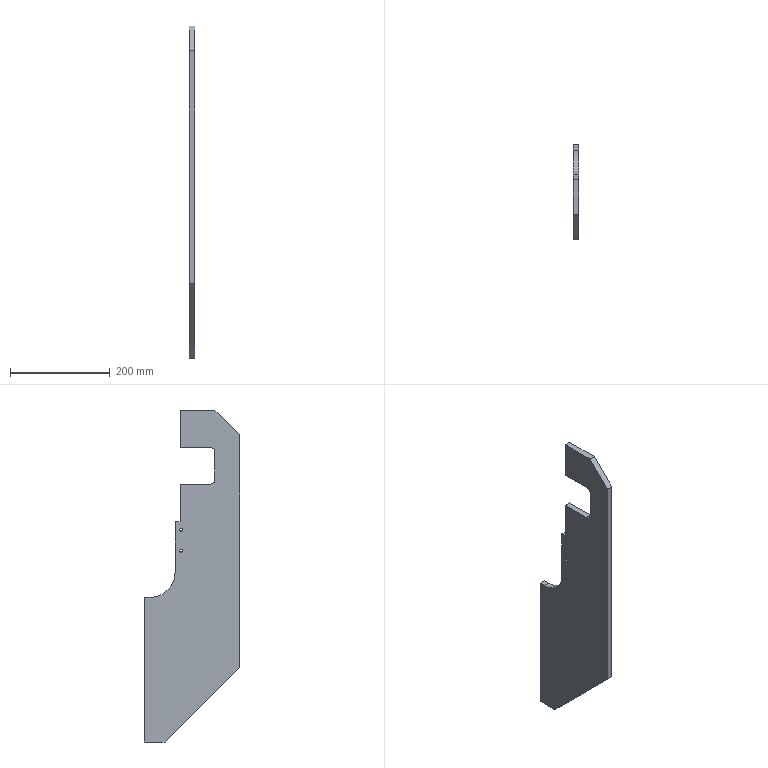Part | STEP file | CENTERING.RIB.2.stp | 1 solid | 49 faces | box 12 x 192 x 666 mm | volume 1019240 mm3 | spline 17 | plane 17 | cylinder 15 | commonest cylinder face diameters 6 x10 20 x4 100 x1